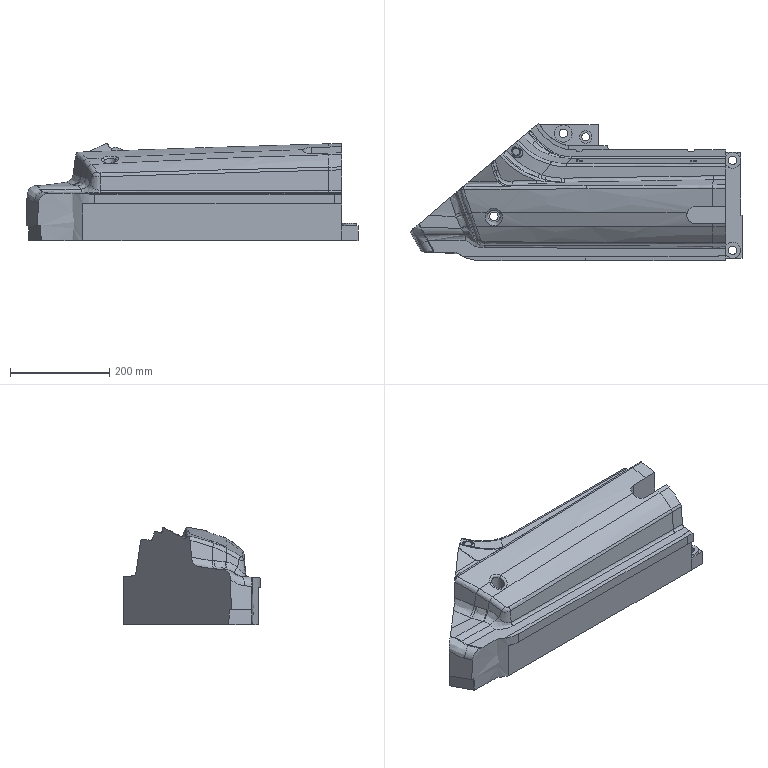Part | NX | features solid 2 | 1 solid | 169 faces | box 669.082 x 276.897 x 195.976 mm | volume 15915785 mm3 | spline 117 | plane 36 | cylinder 16 | commonest cylinder face diameters 17 x4 40 x4 25 x2 32 x2 35 x2 16 x1